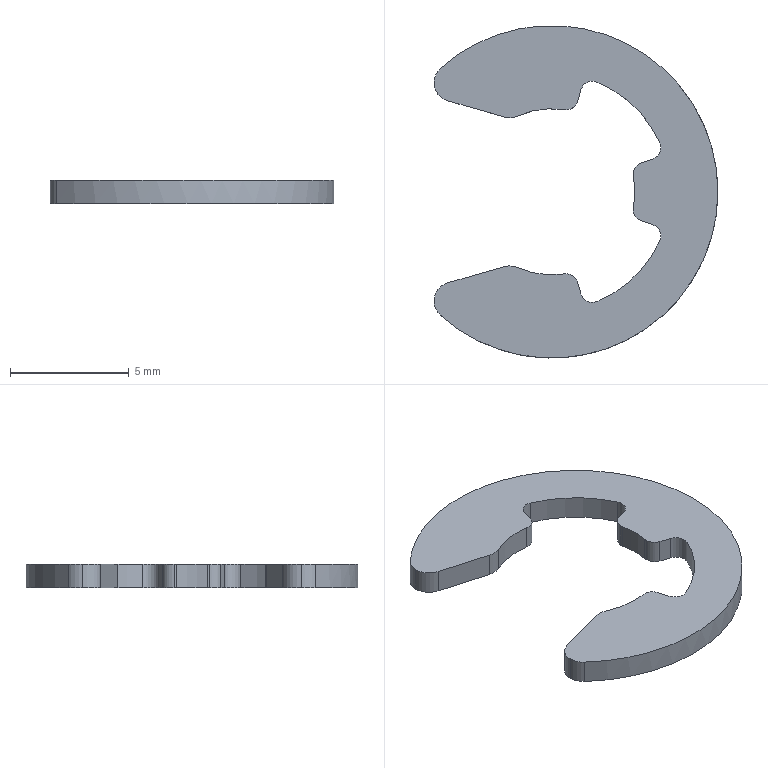Part | STEP file | MSBR-21_1_1_1_1 | 1 solid | 30 faces | box 11.954 x 14 x 1 mm | volume 73.77 mm3 | cylinder 22 | plane 8 | commonest cylinder face diameters 1 x10 1.6 x6 7 x3 10 x2 14 x1
STEP:
#1=CARTESIAN_POINT('',(0.,0.,0.));
#2=DIRECTION('',(0.,0.,1.));
#3=DIRECTION('',(1.,0.,0.));
#4=AXIS2_PLACEMENT_3D('',#1,#2,#3);
#5=CARTESIAN_POINT('',(3.438,0.657,29.2));
#6=VERTEX_POINT('',#5);
#7=CARTESIAN_POINT('',(3.438,-0.657,29.2));
#8=VERTEX_POINT('',#7);
#9=CARTESIAN_POINT('',(-0.000000002,0.000000005,29.2));
#10=DIRECTION('',(0.,0.,-1.));
#11=DIRECTION('',(0.9822,0.1877,0.));
#12=AXIS2_PLACEMENT_3D('',#9,#10,#11);
#13=CIRCLE('',#12,3.5);
#14=EDGE_CURVE('',#6,#8,#13,.T.);
#15=ORIENTED_EDGE('',*,*,#14,.T.);
#16=CARTESIAN_POINT('',(3.429,-0.7508,29.2));
#17=VERTEX_POINT('',#16);
#18=CARTESIAN_POINT('',(3.929,-0.7508,29.2));
#19=DIRECTION('',(0.,0.,1.));
#20=DIRECTION('',(-0.9822,0.1877,0.));
#21=AXIS2_PLACEMENT_3D('',#18,#19,#20);
#22=CIRCLE('',#21,0.5);
#23=EDGE_CURVE('',#8,#17,#22,.T.);
#24=ORIENTED_EDGE('',*,*,#23,.T.);
#25=CARTESIAN_POINT('',(3.774,-1.226,29.2));
#26=VERTEX_POINT('',#25);
#27=CARTESIAN_POINT('',(3.929,-0.7508,29.2));
#28=DIRECTION('',(0.,0.,1.));
#29=DIRECTION('',(-1.,-0.000000003,0.));
#30=AXIS2_PLACEMENT_3D('',#27,#28,#29);
#31=CIRCLE('',#30,0.5);
#32=EDGE_CURVE('',#17,#26,#31,.T.);
#33=ORIENTED_EDGE('',*,*,#32,.T.);
#34=CARTESIAN_POINT('',(4.253,-1.382,29.2));
#35=VERTEX_POINT('',#34);
#36=CARTESIAN_POINT('',(3.774,-1.226,29.2));
#37=DIRECTION('',(0.9511,-0.309,0.));
#38=VECTOR('',#37,0.5035);
#39=LINE('',#36,#38);
#40=EDGE_CURVE('',#26,#35,#39,.T.);
#41=ORIENTED_EDGE('',*,*,#40,.T.);
#42=CARTESIAN_POINT('',(4.554,-2.064,29.2));
#43=VERTEX_POINT('',#42);
#44=CARTESIAN_POINT('',(4.099,-1.857,29.2));
#45=DIRECTION('',(0.,0.,-1.));
#46=DIRECTION('',(0.309,0.9511,0.));
#47=AXIS2_PLACEMENT_3D('',#44,#45,#46);
#48=CIRCLE('',#47,0.5);
#49=EDGE_CURVE('',#35,#43,#48,.T.);
#50=ORIENTED_EDGE('',*,*,#49,.T.);
#51=CARTESIAN_POINT('',(1.904,-4.623,29.2));
#52=VERTEX_POINT('',#51);
#53=CARTESIAN_POINT('',(-0.000000006,0.000000006,29.2));
#54=DIRECTION('',(0.,0.,-1.));
#55=DIRECTION('',(0.9108,-0.4128,0.));
#56=AXIS2_PLACEMENT_3D('',#53,#54,#55);
#57=CIRCLE('',#56,5.);
#58=EDGE_CURVE('',#43,#52,#57,.T.);
#59=ORIENTED_EDGE('',*,*,#58,.T.);
#60=CARTESIAN_POINT('',(1.233,-4.299,29.2));
#61=VERTEX_POINT('',#60);
#62=CARTESIAN_POINT('',(1.713,-4.161,29.2));
#63=DIRECTION('',(0.,0.,-1.));
#64=DIRECTION('',(0.3807,-0.9247,0.));
#65=AXIS2_PLACEMENT_3D('',#62,#63,#64);
#66=CIRCLE('',#65,0.5);
#67=EDGE_CURVE('',#52,#61,#66,.T.);
#68=ORIENTED_EDGE('',*,*,#67,.T.);
#69=CARTESIAN_POINT('',(1.094,-3.815,29.2));
#70=VERTEX_POINT('',#69);
#71=CARTESIAN_POINT('',(1.233,-4.299,29.2));
#72=DIRECTION('',(-0.2756,0.9613,0.));
#73=VECTOR('',#72,0.5035);
#74=LINE('',#71,#73);
#75=EDGE_CURVE('',#61,#70,#74,.T.);
#76=ORIENTED_EDGE('',*,*,#75,.T.);
#77=CARTESIAN_POINT('',(0.5366,-3.459,29.2));
#78=VERTEX_POINT('',#77);
#79=CARTESIAN_POINT('',(0.6133,-3.953,29.2));
#80=DIRECTION('',(0.,0.,1.));
#81=DIRECTION('',(0.9613,0.2756,0.));
#82=AXIS2_PLACEMENT_3D('',#79,#80,#81);
#83=CIRCLE('',#82,0.5);
#84=EDGE_CURVE('',#70,#78,#83,.T.);
#85=ORIENTED_EDGE('',*,*,#84,.T.);
#86=CARTESIAN_POINT('',(-1.44,-3.19,29.2));
#87=VERTEX_POINT('',#86);
#88=CARTESIAN_POINT('',(-0.000000004,0.000000014,29.2));
#89=DIRECTION('',(0.,0.,-1.));
#90=DIRECTION('',(0.1533,-0.9882,0.));
#91=AXIS2_PLACEMENT_3D('',#88,#89,#90);
#92=CIRCLE('',#91,3.5);
#93=EDGE_CURVE('',#78,#87,#92,.T.);
#94=ORIENTED_EDGE('',*,*,#93,.T.);
#95=CARTESIAN_POINT('',(-1.99,-3.15,29.2));
#96=VERTEX_POINT('',#95);
#97=CARTESIAN_POINT('',(-1.77,-3.919,29.2));
#98=DIRECTION('',(0.,0.,1.));
#99=DIRECTION('',(0.4115,0.9114,0.));
#100=AXIS2_PLACEMENT_3D('',#97,#98,#99);
#101=CIRCLE('',#100,0.8);
#102=EDGE_CURVE('',#87,#96,#101,.T.);
#103=ORIENTED_EDGE('',*,*,#102,.T.);
#104=CARTESIAN_POINT('',(-4.374,-3.834,29.2));
#105=VERTEX_POINT('',#104);
#106=CARTESIAN_POINT('',(-1.99,-3.15,29.2));
#107=DIRECTION('',(-0.9613,-0.2756,0.));
#108=VECTOR('',#107,2.48);
#109=LINE('',#106,#108);
#110=EDGE_CURVE('',#96,#105,#109,.T.);
#111=ORIENTED_EDGE('',*,*,#110,.T.);
#112=CARTESIAN_POINT('',(-4.954,-4.603,29.2));
#113=VERTEX_POINT('',#112);
#114=CARTESIAN_POINT('',(-4.154,-4.603,29.2));
#115=DIRECTION('',(0.,0.,1.));
#116=DIRECTION('',(-0.2756,0.9613,0.));
#117=AXIS2_PLACEMENT_3D('',#114,#115,#116);
#118=CIRCLE('',#117,0.8);
#119=EDGE_CURVE('',#105,#113,#118,.T.);
#120=ORIENTED_EDGE('',*,*,#119,.T.);
#121=CARTESIAN_POINT('',(-4.69,-5.197,29.2));
#122=VERTEX_POINT('',#121);
#123=CARTESIAN_POINT('',(-4.154,-4.603,29.2));
#124=DIRECTION('',(0.,0.,1.));
#125=DIRECTION('',(-1.,0.000000001,0.));
#126=AXIS2_PLACEMENT_3D('',#123,#124,#125);
#127=CIRCLE('',#126,0.8);
#128=EDGE_CURVE('',#113,#122,#127,.T.);
#129=ORIENTED_EDGE('',*,*,#128,.T.);
#130=CARTESIAN_POINT('',(4.69,5.197,29.2));
#131=VERTEX_POINT('',#130);
#132=CARTESIAN_POINT('',(-0.000000007,0.000000005,29.2));
#133=DIRECTION('',(0.,0.,1.));
#134=DIRECTION('',(-0.67,-0.7424,0.));
#135=AXIS2_PLACEMENT_3D('',#132,#133,#134);
#136=CIRCLE('',#135,7.);
#137=EDGE_CURVE('',#122,#131,#136,.T.);
#138=ORIENTED_EDGE('',*,*,#137,.T.);
#139=CARTESIAN_POINT('',(-4.69,5.197,29.2));
#140=VERTEX_POINT('',#139);
#141=CARTESIAN_POINT('',(-0.000000007,0.000000005,29.2));
#142=DIRECTION('',(0.,0.,1.));
#143=DIRECTION('',(0.67,0.7424,0.));
#144=AXIS2_PLACEMENT_3D('',#141,#142,#143);
#145=CIRCLE('',#144,7.);
#146=EDGE_CURVE('',#131,#140,#145,.T.);
#147=ORIENTED_EDGE('',*,*,#146,.T.);
#148=CARTESIAN_POINT('',(-4.954,4.603,29.2));
#149=VERTEX_POINT('',#148);
#150=CARTESIAN_POINT('',(-4.154,4.603,29.2));
#151=DIRECTION('',(0.,0.,1.));
#152=DIRECTION('',(-0.67,0.7424,0.));
#153=AXIS2_PLACEMENT_3D('',#150,#151,#152);
#154=CIRCLE('',#153,0.8);
#155=EDGE_CURVE('',#140,#149,#154,.T.);
#156=ORIENTED_EDGE('',*,*,#155,.T.);
#157=CARTESIAN_POINT('',(-4.374,3.834,29.2));
#158=VERTEX_POINT('',#157);
#159=CARTESIAN_POINT('',(-4.154,4.603,29.2));
#160=DIRECTION('',(0.,0.,1.));
#161=DIRECTION('',(-1.,-0.000000001,0.));
#162=AXIS2_PLACEMENT_3D('',#159,#160,#161);
#163=CIRCLE('',#162,0.8);
#164=EDGE_CURVE('',#149,#158,#163,.T.);
#165=ORIENTED_EDGE('',*,*,#164,.T.);
#166=CARTESIAN_POINT('',(-1.99,3.15,29.2));
#167=VERTEX_POINT('',#166);
#168=CARTESIAN_POINT('',(-4.374,3.834,29.2));
#169=DIRECTION('',(0.9613,-0.2756,0.));
#170=VECTOR('',#169,2.48);
#171=LINE('',#168,#170);
#172=EDGE_CURVE('',#158,#167,#171,.T.);
#173=ORIENTED_EDGE('',*,*,#172,.T.);
#174=CARTESIAN_POINT('',(-1.44,3.19,29.2));
#175=VERTEX_POINT('',#174);
#176=CARTESIAN_POINT('',(-1.77,3.919,29.2));
#177=DIRECTION('',(0.,0.,1.));
#178=DIRECTION('',(-0.2756,-0.9613,0.));
#179=AXIS2_PLACEMENT_3D('',#176,#177,#178);
#180=CIRCLE('',#179,0.8);
#181=EDGE_CURVE('',#167,#175,#180,.T.);
#182=ORIENTED_EDGE('',*,*,#181,.T.);
#183=CARTESIAN_POINT('',(0.5366,3.459,29.2));
#184=VERTEX_POINT('',#183);
#185=CARTESIAN_POINT('',(-0.000000004,-0.000000004,29.2));
#186=DIRECTION('',(0.,0.,-1.));
#187=DIRECTION('',(-0.4115,0.9114,0.));
#188=AXIS2_PLACEMENT_3D('',#185,#186,#187);
#189=CIRCLE('',#188,3.5);
#190=EDGE_CURVE('',#175,#184,#189,.T.);
#191=ORIENTED_EDGE('',*,*,#190,.T.);
#192=CARTESIAN_POINT('',(1.094,3.815,29.2));
#193=VERTEX_POINT('',#192);
#194=CARTESIAN_POINT('',(0.6133,3.953,29.2));
#195=DIRECTION('',(0.,0.,1.));
#196=DIRECTION('',(-0.1533,-0.9882,0.));
#197=AXIS2_PLACEMENT_3D('',#194,#195,#196);
#198=CIRCLE('',#197,0.5);
#199=EDGE_CURVE('',#184,#193,#198,.T.);
#200=ORIENTED_EDGE('',*,*,#199,.T.);
#201=CARTESIAN_POINT('',(1.233,4.299,29.2));
#202=VERTEX_POINT('',#201);
#203=CARTESIAN_POINT('',(1.094,3.815,29.2));
#204=DIRECTION('',(0.2756,0.9613,0.));
#205=VECTOR('',#204,0.5035);
#206=LINE('',#203,#205);
#207=EDGE_CURVE('',#193,#202,#206,.T.);
#208=ORIENTED_EDGE('',*,*,#207,.T.);
#209=CARTESIAN_POINT('',(1.904,4.623,29.2));
#210=VERTEX_POINT('',#209);
#211=CARTESIAN_POINT('',(1.713,4.161,29.2));
#212=DIRECTION('',(0.,0.,-1.));
#213=DIRECTION('',(-0.9613,0.2756,0.));
#214=AXIS2_PLACEMENT_3D('',#211,#212,#213);
#215=CIRCLE('',#214,0.5);
#216=EDGE_CURVE('',#202,#210,#215,.T.);
#217=ORIENTED_EDGE('',*,*,#216,.T.);
#218=CARTESIAN_POINT('',(4.554,2.064,29.2));
#219=VERTEX_POINT('',#218);
#220=CARTESIAN_POINT('',(-0.000000006,0.000000004,29.2));
#221=DIRECTION('',(0.,0.,-1.));
#222=DIRECTION('',(0.3807,0.9247,0.));
#223=AXIS2_PLACEMENT_3D('',#220,#221,#222);
#224=CIRCLE('',#223,5.);
#225=EDGE_CURVE('',#210,#219,#224,.T.);
#226=ORIENTED_EDGE('',*,*,#225,.T.);
#227=CARTESIAN_POINT('',(4.253,1.382,29.2));
#228=VERTEX_POINT('',#227);
#229=CARTESIAN_POINT('',(4.099,1.857,29.2));
#230=DIRECTION('',(0.,0.,-1.));
#231=DIRECTION('',(0.9108,0.4128,0.));
#232=AXIS2_PLACEMENT_3D('',#229,#230,#231);
#233=CIRCLE('',#232,0.5);
#234=EDGE_CURVE('',#219,#228,#233,.T.);
#235=ORIENTED_EDGE('',*,*,#234,.T.);
#236=CARTESIAN_POINT('',(3.774,1.226,29.2));
#237=VERTEX_POINT('',#236);
#238=CARTESIAN_POINT('',(4.253,1.382,29.2));
#239=DIRECTION('',(-0.9511,-0.309,0.));
#240=VECTOR('',#239,0.5035);
#241=LINE('',#238,#240);
#242=EDGE_CURVE('',#228,#237,#241,.T.);
#243=ORIENTED_EDGE('',*,*,#242,.T.);
#244=CARTESIAN_POINT('',(3.429,0.7508,29.2));
#245=VERTEX_POINT('',#244);
#246=CARTESIAN_POINT('',(3.929,0.7508,29.2));
#247=DIRECTION('',(0.,0.,1.));
#248=DIRECTION('',(-0.309,0.9511,0.));
#249=AXIS2_PLACEMENT_3D('',#246,#247,#248);
#250=CIRCLE('',#249,0.5);
#251=EDGE_CURVE('',#237,#245,#250,.T.);
#252=ORIENTED_EDGE('',*,*,#251,.T.);
#253=CARTESIAN_POINT('',(3.929,0.7508,29.2));
#254=DIRECTION('',(0.,0.,1.));
#255=DIRECTION('',(-1.,-0.000000007,0.));
#256=AXIS2_PLACEMENT_3D('',#253,#254,#255);
#257=CIRCLE('',#256,0.5);
#258=EDGE_CURVE('',#245,#6,#257,.T.);
#259=ORIENTED_EDGE('',*,*,#258,.T.);
#260=EDGE_LOOP('',(#15,#24,#33,#41,#50,#59,#68,#76,#85,#94,#103,#111,#120,#129,#138,#147,#156,#165,#173,#182,#191,#200,#208,#217,#226,#235,#243,#252,#259));
#261=FACE_OUTER_BOUND('',#260,.F.);
#262=CARTESIAN_POINT('',(1.025,0.000002085,29.2));
#263=DIRECTION('',(0.,0.,1.));
#264=DIRECTION('',(0.,1.,0.));
#265=AXIS2_PLACEMENT_3D('',#262,#263,#264);
#266=PLANE('',#265);
#267=ADVANCED_FACE('',(#261),#266,.F.);
#268=CARTESIAN_POINT('',(3.438,-0.657,30.2));
#269=VERTEX_POINT('',#268);
#270=CARTESIAN_POINT('',(3.438,0.657,30.2));
#271=VERTEX_POINT('',#270);
#272=CARTESIAN_POINT('',(-0.000000002,0.000000005,30.2));
#273=DIRECTION('',(0.,0.,1.));
#274=DIRECTION('',(0.9822,-0.1877,0.));
#275=AXIS2_PLACEMENT_3D('',#272,#273,#274);
#276=CIRCLE('',#275,3.5);
#277=EDGE_CURVE('',#269,#271,#276,.T.);
#278=ORIENTED_EDGE('',*,*,#277,.F.);
#279=CARTESIAN_POINT('',(3.438,-0.657,29.2));
#280=DIRECTION('',(0.,0.,1.));
#281=VECTOR('',#280,1.);
#282=LINE('',#279,#281);
#283=EDGE_CURVE('',#8,#269,#282,.T.);
#284=ORIENTED_EDGE('',*,*,#283,.F.);
#285=ORIENTED_EDGE('',*,*,#14,.F.);
#286=CARTESIAN_POINT('',(3.438,0.657,30.2));
#287=DIRECTION('',(0.,0.,-1.));
#288=VECTOR('',#287,1.);
#289=LINE('',#286,#288);
#290=EDGE_CURVE('',#271,#6,#289,.T.);
#291=ORIENTED_EDGE('',*,*,#290,.F.);
#292=EDGE_LOOP('',(#278,#284,#285,#291));
#293=FACE_OUTER_BOUND('',#292,.F.);
#294=CARTESIAN_POINT('',(-0.000000002,0.000000005,29.178));
#295=DIRECTION('',(0.,0.,1.));
#296=DIRECTION('',(0.9822,-0.1877,0.));
#297=AXIS2_PLACEMENT_3D('',#294,#295,#296);
#298=CYLINDRICAL_SURFACE('',#297,3.5);
#299=ADVANCED_FACE('',(#293),#298,.F.);
#300=CARTESIAN_POINT('',(4.253,-1.382,30.2));
#301=VERTEX_POINT('',#300);
#302=CARTESIAN_POINT('',(3.774,-1.226,30.2));
#303=VERTEX_POINT('',#302);
#304=CARTESIAN_POINT('',(4.253,-1.382,30.2));
#305=DIRECTION('',(-0.9511,0.309,0.));
#306=VECTOR('',#305,0.5035);
#307=LINE('',#304,#306);
#308=EDGE_CURVE('',#301,#303,#307,.T.);
#309=ORIENTED_EDGE('',*,*,#308,.T.);
#310=CARTESIAN_POINT('',(3.429,-0.7508,30.2));
#311=VERTEX_POINT('',#310);
#312=CARTESIAN_POINT('',(3.929,-0.7508,30.2));
#313=DIRECTION('',(0.,0.,-1.));
#314=DIRECTION('',(-0.309,-0.9511,0.));
#315=AXIS2_PLACEMENT_3D('',#312,#313,#314);
#316=CIRCLE('',#315,0.5);
#317=EDGE_CURVE('',#303,#311,#316,.T.);
#318=ORIENTED_EDGE('',*,*,#317,.T.);
#319=CARTESIAN_POINT('',(3.929,-0.7508,30.2));
#320=DIRECTION('',(0.,0.,-1.));
#321=DIRECTION('',(-1.,0.000000007,0.));
#322=AXIS2_PLACEMENT_3D('',#319,#320,#321);
#323=CIRCLE('',#322,0.5);
#324=EDGE_CURVE('',#311,#269,#323,.T.);
#325=ORIENTED_EDGE('',*,*,#324,.T.);
#326=ORIENTED_EDGE('',*,*,#277,.T.);
#327=CARTESIAN_POINT('',(3.429,0.7508,30.2));
#328=VERTEX_POINT('',#327);
#329=CARTESIAN_POINT('',(3.929,0.7508,30.2));
#330=DIRECTION('',(0.,0.,-1.));
#331=DIRECTION('',(-0.9822,-0.1877,0.));
#332=AXIS2_PLACEMENT_3D('',#329,#330,#331);
#333=CIRCLE('',#332,0.5);
#334=EDGE_CURVE('',#271,#328,#333,.T.);
#335=ORIENTED_EDGE('',*,*,#334,.T.);
#336=CARTESIAN_POINT('',(3.774,1.226,30.2));
#337=VERTEX_POINT('',#336);
#338=CARTESIAN_POINT('',(3.929,0.7508,30.2));
#339=DIRECTION('',(0.,0.,-1.));
#340=DIRECTION('',(-1.,0.000000003,0.));
#341=AXIS2_PLACEMENT_3D('',#338,#339,#340);
#342=CIRCLE('',#341,0.5);
#343=EDGE_CURVE('',#328,#337,#342,.T.);
#344=ORIENTED_EDGE('',*,*,#343,.T.);
#345=CARTESIAN_POINT('',(4.253,1.382,30.2));
#346=VERTEX_POINT('',#345);
#347=CARTESIAN_POINT('',(3.774,1.226,30.2));
#348=DIRECTION('',(0.9511,0.309,0.));
#349=VECTOR('',#348,0.5035);
#350=LINE('',#347,#349);
#351=EDGE_CURVE('',#337,#346,#350,.T.);
#352=ORIENTED_EDGE('',*,*,#351,.T.);
#353=CARTESIAN_POINT('',(4.554,2.064,30.2));
#354=VERTEX_POINT('',#353);
#355=CARTESIAN_POINT('',(4.099,1.857,30.2));
#356=DIRECTION('',(0.,0.,1.));
#357=DIRECTION('',(0.309,-0.9511,0.));
#358=AXIS2_PLACEMENT_3D('',#355,#356,#357);
#359=CIRCLE('',#358,0.5);
#360=EDGE_CURVE('',#346,#354,#359,.T.);
#361=ORIENTED_EDGE('',*,*,#360,.T.);
#362=CARTESIAN_POINT('',(1.904,4.623,30.2));
#363=VERTEX_POINT('',#362);
#364=CARTESIAN_POINT('',(-0.000000006,0.000000004,30.2));
#365=DIRECTION('',(0.,0.,1.));
#366=DIRECTION('',(0.9108,0.4128,0.));
#367=AXIS2_PLACEMENT_3D('',#364,#365,#366);
#368=CIRCLE('',#367,5.);
#369=EDGE_CURVE('',#354,#363,#368,.T.);
#370=ORIENTED_EDGE('',*,*,#369,.T.);
#371=CARTESIAN_POINT('',(1.233,4.299,30.2));
#372=VERTEX_POINT('',#371);
#373=CARTESIAN_POINT('',(1.713,4.161,30.2));
#374=DIRECTION('',(0.,0.,1.));
#375=DIRECTION('',(0.3807,0.9247,0.));
#376=AXIS2_PLACEMENT_3D('',#373,#374,#375);
#377=CIRCLE('',#376,0.5);
#378=EDGE_CURVE('',#363,#372,#377,.T.);
#379=ORIENTED_EDGE('',*,*,#378,.T.);
#380=CARTESIAN_POINT('',(1.094,3.815,30.2));
#381=VERTEX_POINT('',#380);
#382=CARTESIAN_POINT('',(1.233,4.299,30.2));
#383=DIRECTION('',(-0.2756,-0.9613,0.));
#384=VECTOR('',#383,0.5035);
#385=LINE('',#382,#384);
#386=EDGE_CURVE('',#372,#381,#385,.T.);
#387=ORIENTED_EDGE('',*,*,#386,.T.);
#388=CARTESIAN_POINT('',(0.5366,3.459,30.2));
#389=VERTEX_POINT('',#388);
#390=CARTESIAN_POINT('',(0.6133,3.953,30.2));
#391=DIRECTION('',(0.,0.,-1.));
#392=DIRECTION('',(0.9613,-0.2756,0.));
#393=AXIS2_PLACEMENT_3D('',#390,#391,#392);
#394=CIRCLE('',#393,0.5);
#395=EDGE_CURVE('',#381,#389,#394,.T.);
#396=ORIENTED_EDGE('',*,*,#395,.T.);
#397=CARTESIAN_POINT('',(-1.44,3.19,30.2));
#398=VERTEX_POINT('',#397);
#399=CARTESIAN_POINT('',(-0.000000004,-0.000000004,30.2));
#400=DIRECTION('',(0.,0.,1.));
#401=DIRECTION('',(0.1533,0.9882,0.));
#402=AXIS2_PLACEMENT_3D('',#399,#400,#401);
#403=CIRCLE('',#402,3.5);
#404=EDGE_CURVE('',#389,#398,#403,.T.);
#405=ORIENTED_EDGE('',*,*,#404,.T.);
#406=CARTESIAN_POINT('',(-1.99,3.15,30.2));
#407=VERTEX_POINT('',#406);
#408=CARTESIAN_POINT('',(-1.77,3.919,30.2));
#409=DIRECTION('',(0.,0.,-1.));
#410=DIRECTION('',(0.4115,-0.9114,0.));
#411=AXIS2_PLACEMENT_3D('',#408,#409,#410);
#412=CIRCLE('',#411,0.8);
#413=EDGE_CURVE('',#398,#407,#412,.T.);
#414=ORIENTED_EDGE('',*,*,#413,.T.);
#415=CARTESIAN_POINT('',(-4.374,3.834,30.2));
#416=VERTEX_POINT('',#415);
#417=CARTESIAN_POINT('',(-1.99,3.15,30.2));
#418=DIRECTION('',(-0.9613,0.2756,0.));
#419=VECTOR('',#418,2.48);
#420=LINE('',#417,#419);
#421=EDGE_CURVE('',#407,#416,#420,.T.);
#422=ORIENTED_EDGE('',*,*,#421,.T.);
#423=CARTESIAN_POINT('',(-4.954,4.603,30.2));
#424=VERTEX_POINT('',#423);
#425=CARTESIAN_POINT('',(-4.154,4.603,30.2));
#426=DIRECTION('',(0.,0.,-1.));
#427=DIRECTION('',(-0.2756,-0.9613,0.));
#428=AXIS2_PLACEMENT_3D('',#425,#426,#427);
#429=CIRCLE('',#428,0.8);
#430=EDGE_CURVE('',#416,#424,#429,.T.);
#431=ORIENTED_EDGE('',*,*,#430,.T.);
#432=CARTESIAN_POINT('',(-4.69,5.197,30.2));
#433=VERTEX_POINT('',#432);
#434=CARTESIAN_POINT('',(-4.154,4.603,30.2));
#435=DIRECTION('',(0.,0.,-1.));
#436=DIRECTION('',(-1.,-0.000000001,0.));
#437=AXIS2_PLACEMENT_3D('',#434,#435,#436);
#438=CIRCLE('',#437,0.8);
#439=EDGE_CURVE('',#424,#433,#438,.T.);
#440=ORIENTED_EDGE('',*,*,#439,.T.);
#441=CARTESIAN_POINT('',(4.69,5.197,30.2));
#442=VERTEX_POINT('',#441);
#443=CARTESIAN_POINT('',(-0.000000007,0.000000005,30.2));
#444=DIRECTION('',(0.,0.,-1.));
#445=DIRECTION('',(-0.67,0.7424,0.));
#446=AXIS2_PLACEMENT_3D('',#443,#444,#445);
#447=CIRCLE('',#446,7.);
#448=EDGE_CURVE('',#433,#442,#447,.T.);
#449=ORIENTED_EDGE('',*,*,#448,.T.);
#450=CARTESIAN_POINT('',(4.69,-5.197,30.2));
#451=VERTEX_POINT('',#450);
#452=CARTESIAN_POINT('',(-0.000000007,0.000000005,30.2));
#453=DIRECTION('',(0.,0.,-1.));
#454=DIRECTION('',(0.67,0.7424,0.));
#455=AXIS2_PLACEMENT_3D('',#452,#453,#454);
#456=CIRCLE('',#455,7.);
#457=EDGE_CURVE('',#442,#451,#456,.T.);
#458=ORIENTED_EDGE('',*,*,#457,.T.);
#459=CARTESIAN_POINT('',(-4.69,-5.197,30.2));
#460=VERTEX_POINT('',#459);
#461=CARTESIAN_POINT('',(-0.000000007,0.000000005,30.2));
#462=DIRECTION('',(0.,0.,-1.));
#463=DIRECTION('',(0.67,-0.7424,0.));
#464=AXIS2_PLACEMENT_3D('',#461,#462,#463);
#465=CIRCLE('',#464,7.);
#466=EDGE_CURVE('',#451,#460,#465,.T.);
#467=ORIENTED_EDGE('',*,*,#466,.T.);
#468=CARTESIAN_POINT('',(-4.954,-4.603,30.2));
#469=VERTEX_POINT('',#468);
#470=CARTESIAN_POINT('',(-4.154,-4.603,30.2));
#471=DIRECTION('',(0.,0.,-1.));
#472=DIRECTION('',(-0.67,-0.7424,0.));
#473=AXIS2_PLACEMENT_3D('',#470,#471,#472);
#474=CIRCLE('',#473,0.8);
#475=EDGE_CURVE('',#460,#469,#474,.T.);
#476=ORIENTED_EDGE('',*,*,#475,.T.);
#477=CARTESIAN_POINT('',(-4.374,-3.834,30.2));
#478=VERTEX_POINT('',#477);
#479=CARTESIAN_POINT('',(-4.154,-4.603,30.2));
#480=DIRECTION('',(0.,0.,-1.));
#481=DIRECTION('',(-1.,0.000000001,0.));
#482=AXIS2_PLACEMENT_3D('',#479,#480,#481);
#483=CIRCLE('',#482,0.8);
#484=EDGE_CURVE('',#469,#478,#483,.T.);
#485=ORIENTED_EDGE('',*,*,#484,.T.);
#486=CARTESIAN_POINT('',(-1.99,-3.15,30.2));
#487=VERTEX_POINT('',#486);
#488=CARTESIAN_POINT('',(-4.374,-3.834,30.2));
#489=DIRECTION('',(0.9613,0.2756,0.));
#490=VECTOR('',#489,2.48);
#491=LINE('',#488,#490);
#492=EDGE_CURVE('',#478,#487,#491,.T.);
#493=ORIENTED_EDGE('',*,*,#492,.T.);
#494=CARTESIAN_POINT('',(-1.44,-3.19,30.2));
#495=VERTEX_POINT('',#494);
#496=CARTESIAN_POINT('',(-1.77,-3.919,30.2));
#497=DIRECTION('',(0.,0.,-1.));
#498=DIRECTION('',(-0.2756,0.9613,0.));
#499=AXIS2_PLACEMENT_3D('',#496,#497,#498);
#500=CIRCLE('',#499,0.8);
#501=EDGE_CURVE('',#487,#495,#500,.T.);
#502=ORIENTED_EDGE('',*,*,#501,.T.);
#503=CARTESIAN_POINT('',(0.5366,-3.459,30.2));
#504=VERTEX_POINT('',#503);
#505=CARTESIAN_POINT('',(-0.000000004,0.000000014,30.2));
#506=DIRECTION('',(0.,0.,1.));
#507=DIRECTION('',(-0.4115,-0.9114,0.));
#508=AXIS2_PLACEMENT_3D('',#505,#506,#507);
#509=CIRCLE('',#508,3.5);
#510=EDGE_CURVE('',#495,#504,#509,.T.);
#511=ORIENTED_EDGE('',*,*,#510,.T.);
#512=CARTESIAN_POINT('',(1.094,-3.815,30.2));
#513=VERTEX_POINT('',#512);
#514=CARTESIAN_POINT('',(0.6133,-3.953,30.2));
#515=DIRECTION('',(0.,0.,-1.));
#516=DIRECTION('',(-0.1533,0.9882,0.));
#517=AXIS2_PLACEMENT_3D('',#514,#515,#516);
#518=CIRCLE('',#517,0.5);
#519=EDGE_CURVE('',#504,#513,#518,.T.);
#520=ORIENTED_EDGE('',*,*,#519,.T.);
#521=CARTESIAN_POINT('',(1.233,-4.299,30.2));
#522=VERTEX_POINT('',#521);
#523=CARTESIAN_POINT('',(1.094,-3.815,30.2));
#524=DIRECTION('',(0.2756,-0.9613,0.));
#525=VECTOR('',#524,0.5035);
#526=LINE('',#523,#525);
#527=EDGE_CURVE('',#513,#522,#526,.T.);
#528=ORIENTED_EDGE('',*,*,#527,.T.);
#529=CARTESIAN_POINT('',(1.904,-4.623,30.2));
#530=VERTEX_POINT('',#529);
#531=CARTESIAN_POINT('',(1.713,-4.161,30.2));
#532=DIRECTION('',(0.,0.,1.));
#533=DIRECTION('',(-0.9613,-0.2756,0.));
#534=AXIS2_PLACEMENT_3D('',#531,#532,#533);
#535=CIRCLE('',#534,0.5);
#536=EDGE_CURVE('',#522,#530,#535,.T.);
#537=ORIENTED_EDGE('',*,*,#536,.T.);
#538=CARTESIAN_POINT('',(4.554,-2.064,30.2));
#539=VERTEX_POINT('',#538);
#540=CARTESIAN_POINT('',(-0.000000006,0.000000006,30.2));
#541=DIRECTION('',(0.,0.,1.));
#542=DIRECTION('',(0.3807,-0.9247,0.));
#543=AXIS2_PLACEMENT_3D('',#540,#541,#542);
#544=CIRCLE('',#543,5.);
#545=EDGE_CURVE('',#530,#539,#544,.T.);
#546=ORIENTED_EDGE('',*,*,#545,.T.);
#547=CARTESIAN_POINT('',(4.099,-1.857,30.2));
#548=DIRECTION('',(0.,0.,1.));
#549=DIRECTION('',(0.9108,-0.4128,0.));
#550=AXIS2_PLACEMENT_3D('',#547,#548,#549);
#551=CIRCLE('',#550,0.5);
#552=EDGE_CURVE('',#539,#301,#551,.T.);
#553=ORIENTED_EDGE('',*,*,#552,.T.);
#554=EDGE_LOOP('',(#309,#318,#325,#326,#335,#344,#352,#361,#370,#379,#387,#396,#405,#414,#422,#431,#440,#449,#458,#467,#476,#485,#493,#502,#511,#520,#528,#537,#546,#553));
#555=FACE_OUTER_BOUND('',#554,.F.);
#556=CARTESIAN_POINT('',(1.025,-0.000002076,30.2));
#557=DIRECTION('',(0.,0.,1.));
#558=DIRECTION('',(0.,1.,0.));
#559=AXIS2_PLACEMENT_3D('',#556,#557,#558);
#560=PLANE('',#559);
#561=ADVANCED_FACE('',(#555),#560,.T.);
#562=ORIENTED_EDGE('',*,*,#40,.F.);
#563=CARTESIAN_POINT('',(3.774,-1.226,30.2));
#564=DIRECTION('',(0.000000001,0.,-1.));
#565=VECTOR('',#564,1.);
#566=LINE('',#563,#565);
#567=EDGE_CURVE('',#303,#26,#566,.T.);
#568=ORIENTED_EDGE('',*,*,#567,.F.);
#569=ORIENTED_EDGE('',*,*,#308,.F.);
#570=CARTESIAN_POINT('',(4.253,-1.382,29.2));
#571=DIRECTION('',(0.,0.,1.));
#572=VECTOR('',#571,1.);
#573=LINE('',#570,#572);
#574=EDGE_CURVE('',#35,#301,#573,.T.);
#575=ORIENTED_EDGE('',*,*,#574,.F.);
#576=EDGE_LOOP('',(#562,#568,#569,#575));
#577=FACE_OUTER_BOUND('',#576,.F.);
#578=CARTESIAN_POINT('',(4.014,-1.304,29.7));
#579=DIRECTION('',(0.309,0.9511,0.));
#580=DIRECTION('',(0.9511,-0.309,0.));
#581=AXIS2_PLACEMENT_3D('',#578,#579,#580);
#582=PLANE('',#581);
#583=ADVANCED_FACE('',(#577),#582,.F.);
#584=ORIENTED_EDGE('',*,*,#567,.T.);
#585=ORIENTED_EDGE('',*,*,#32,.F.);
#586=CARTESIAN_POINT('',(3.429,-0.7508,30.2));
#587=DIRECTION('',(0.,0.,-1.));
#588=VECTOR('',#587,1.);
#589=LINE('',#586,#588);
#590=EDGE_CURVE('',#311,#17,#589,.T.);
#591=ORIENTED_EDGE('',*,*,#590,.F.);
#592=ORIENTED_EDGE('',*,*,#317,.F.);
#593=EDGE_LOOP('',(#584,#585,#591,#592));
#594=FACE_OUTER_BOUND('',#593,.F.);
#595=CARTESIAN_POINT('',(3.929,-0.7508,29.178));
#596=DIRECTION('',(0.,0.,1.));
#597=DIRECTION('',(-1.,-0.000000002,0.));
#598=AXIS2_PLACEMENT_3D('',#595,#596,#597);
#599=CYLINDRICAL_SURFACE('',#598,0.5);
#600=ADVANCED_FACE('',(#594),#599,.T.);
#601=ORIENTED_EDGE('',*,*,#324,.F.);
#602=ORIENTED_EDGE('',*,*,#590,.T.);
#603=ORIENTED_EDGE('',*,*,#23,.F.);
#604=ORIENTED_EDGE('',*,*,#283,.T.);
#605=EDGE_LOOP('',(#601,#602,#603,#604));
#606=FACE_OUTER_BOUND('',#605,.F.);
#607=CARTESIAN_POINT('',(3.929,-0.7508,29.178));
#608=DIRECTION('',(0.,0.,1.));
#609=DIRECTION('',(-0.9822,0.1877,0.));
#610=AXIS2_PLACEMENT_3D('',#607,#608,#609);
#611=CYLINDRICAL_SURFACE('',#610,0.5);
#612=ADVANCED_FACE('',(#606),#611,.T.);
#613=ORIENTED_EDGE('',*,*,#552,.F.);
#614=CARTESIAN_POINT('',(4.554,-2.064,29.2));
#615=DIRECTION('',(0.,0.,1.));
#616=VECTOR('',#615,1.);
#617=LINE('',#614,#616);
#618=EDGE_CURVE('',#43,#539,#617,.T.);
#619=ORIENTED_EDGE('',*,*,#618,.F.);
#620=ORIENTED_EDGE('',*,*,#49,.F.);
#621=ORIENTED_EDGE('',*,*,#574,.T.);
#622=EDGE_LOOP('',(#613,#619,#620,#621));
#623=FACE_OUTER_BOUND('',#622,.F.);
#624=CARTESIAN_POINT('',(4.099,-1.857,29.178));
#625=DIRECTION('',(0.,0.,1.));
#626=DIRECTION('',(0.9108,-0.4128,0.));
#627=AXIS2_PLACEMENT_3D('',#624,#625,#626);
#628=CYLINDRICAL_SURFACE('',#627,0.5);
#629=ADVANCED_FACE('',(#623),#628,.F.);
#630=ORIENTED_EDGE('',*,*,#545,.F.);
#631=CARTESIAN_POINT('',(1.904,-4.623,29.2));
#632=DIRECTION('',(0.,0.,1.));
#633=VECTOR('',#632,1.);
#634=LINE('',#631,#633);
#635=EDGE_CURVE('',#52,#530,#634,.T.);
#636=ORIENTED_EDGE('',*,*,#635,.F.);
#637=ORIENTED_EDGE('',*,*,#58,.F.);
#638=ORIENTED_EDGE('',*,*,#618,.T.);
#639=EDGE_LOOP('',(#630,#636,#637,#638));
#640=FACE_OUTER_BOUND('',#639,.F.);
#641=CARTESIAN_POINT('',(-0.000000006,0.000000006,29.178));
#642=DIRECTION('',(0.,0.,1.));
#643=DIRECTION('',(0.3807,-0.9247,0.));
#644=AXIS2_PLACEMENT_3D('',#641,#642,#643);
#645=CYLINDRICAL_SURFACE('',#644,5.);
#646=ADVANCED_FACE('',(#640),#645,.F.);
#647=ORIENTED_EDGE('',*,*,#536,.F.);
#648=CARTESIAN_POINT('',(1.233,-4.299,30.2));
#649=DIRECTION('',(0.,0.,-1.));
#650=VECTOR('',#649,1.);
#651=LINE('',#648,#650);
#652=EDGE_CURVE('',#522,#61,#651,.T.);
#653=ORIENTED_EDGE('',*,*,#652,.T.);
#654=ORIENTED_EDGE('',*,*,#67,.F.);
#655=ORIENTED_EDGE('',*,*,#635,.T.);
#656=EDGE_LOOP('',(#647,#653,#654,#655));
#657=FACE_OUTER_BOUND('',#656,.F.);
#658=CARTESIAN_POINT('',(1.713,-4.161,29.178));
#659=DIRECTION('',(0.,0.,1.));
#660=DIRECTION('',(-0.9613,-0.2756,0.));
#661=AXIS2_PLACEMENT_3D('',#658,#659,#660);
#662=CYLINDRICAL_SURFACE('',#661,0.5);
#663=ADVANCED_FACE('',(#657),#662,.F.);
#664=ORIENTED_EDGE('',*,*,#75,.F.);
#665=ORIENTED_EDGE('',*,*,#652,.F.);
#666=ORIENTED_EDGE('',*,*,#527,.F.);
#667=CARTESIAN_POINT('',(1.094,-3.815,29.2));
#668=DIRECTION('',(0.,0.,1.));
#669=VECTOR('',#668,1.);
#670=LINE('',#667,#669);
#671=EDGE_CURVE('',#70,#513,#670,.T.);
#672=ORIENTED_EDGE('',*,*,#671,.F.);
#673=EDGE_LOOP('',(#664,#665,#666,#672));
#674=FACE_OUTER_BOUND('',#673,.F.);
#675=CARTESIAN_POINT('',(1.163,-4.057,29.7));
#676=DIRECTION('',(0.9613,0.2756,0.));
#677=DIRECTION('',(-0.2756,0.9613,0.));
#678=AXIS2_PLACEMENT_3D('',#675,#676,#677);
#679=PLANE('',#678);
#680=ADVANCED_FACE('',(#674),#679,.T.);
#681=ORIENTED_EDGE('',*,*,#84,.F.);
#682=ORIENTED_EDGE('',*,*,#671,.T.);
#683=ORIENTED_EDGE('',*,*,#519,.F.);
#684=CARTESIAN_POINT('',(0.5366,-3.459,29.2));
#685=DIRECTION('',(0.,0.,1.));
#686=VECTOR('',#685,1.);
#687=LINE('',#684,#686);
#688=EDGE_CURVE('',#78,#504,#687,.T.);
#689=ORIENTED_EDGE('',*,*,#688,.F.);
#690=EDGE_LOOP('',(#681,#682,#683,#689));
#691=FACE_OUTER_BOUND('',#690,.F.);
#692=CARTESIAN_POINT('',(0.6133,-3.953,29.178));
#693=DIRECTION('',(0.,0.,1.));
#694=DIRECTION('',(0.9613,0.2756,0.));
#695=AXIS2_PLACEMENT_3D('',#692,#693,#694);
#696=CYLINDRICAL_SURFACE('',#695,0.5);
#697=ADVANCED_FACE('',(#691),#696,.T.);
#698=ORIENTED_EDGE('',*,*,#510,.F.);
#699=CARTESIAN_POINT('',(-1.44,-3.19,29.2));
#700=DIRECTION('',(0.,0.,1.));
#701=VECTOR('',#700,1.);
#702=LINE('',#699,#701);
#703=EDGE_CURVE('',#87,#495,#702,.T.);
#704=ORIENTED_EDGE('',*,*,#703,.F.);
#705=ORIENTED_EDGE('',*,*,#93,.F.);
#706=ORIENTED_EDGE('',*,*,#688,.T.);
#707=EDGE_LOOP('',(#698,#704,#705,#706));
#708=FACE_OUTER_BOUND('',#707,.F.);
#709=CARTESIAN_POINT('',(-0.000000004,0.000000014,29.178));
#710=DIRECTION('',(0.,0.,1.));
#711=DIRECTION('',(-0.4115,-0.9114,0.));
#712=AXIS2_PLACEMENT_3D('',#709,#710,#711);
#713=CYLINDRICAL_SURFACE('',#712,3.5);
#714=ADVANCED_FACE('',(#708),#713,.F.);
#715=ORIENTED_EDGE('',*,*,#102,.F.);
#716=ORIENTED_EDGE('',*,*,#703,.T.);
#717=ORIENTED_EDGE('',*,*,#501,.F.);
#718=CARTESIAN_POINT('',(-1.99,-3.15,30.2));
#719=DIRECTION('',(0.,0.,-1.));
#720=VECTOR('',#719,1.);
#721=LINE('',#718,#720);
#722=EDGE_CURVE('',#487,#96,#721,.T.);
#723=ORIENTED_EDGE('',*,*,#722,.T.);
#724=EDGE_LOOP('',(#715,#716,#717,#723));
#725=FACE_OUTER_BOUND('',#724,.F.);
#726=CARTESIAN_POINT('',(-1.77,-3.919,29.178));
#727=DIRECTION('',(0.,0.,1.));
#728=DIRECTION('',(0.4115,0.9114,0.));
#729=AXIS2_PLACEMENT_3D('',#726,#727,#728);
#730=CYLINDRICAL_SURFACE('',#729,0.8);
#731=ADVANCED_FACE('',(#725),#730,.T.);
#732=ORIENTED_EDGE('',*,*,#110,.F.);
#733=ORIENTED_EDGE('',*,*,#722,.F.);
#734=ORIENTED_EDGE('',*,*,#492,.F.);
#735=CARTESIAN_POINT('',(-4.374,-3.834,29.2));
#736=DIRECTION('',(0.,0.,1.));
#737=VECTOR('',#736,1.);
#738=LINE('',#735,#737);
#739=EDGE_CURVE('',#105,#478,#738,.T.);
#740=ORIENTED_EDGE('',*,*,#739,.F.);
#741=EDGE_LOOP('',(#732,#733,#734,#740));
#742=FACE_OUTER_BOUND('',#741,.F.);
#743=CARTESIAN_POINT('',(-3.182,-3.492,29.7));
#744=DIRECTION('',(-0.2756,0.9613,0.));
#745=DIRECTION('',(-0.9613,-0.2756,0.));
#746=AXIS2_PLACEMENT_3D('',#743,#744,#745);
#747=PLANE('',#746);
#748=ADVANCED_FACE('',(#742),#747,.T.);
#749=ORIENTED_EDGE('',*,*,#484,.F.);
#750=CARTESIAN_POINT('',(-4.954,-4.603,29.2));
#751=DIRECTION('',(0.,0.,1.));
#752=VECTOR('',#751,1.);
#753=LINE('',#750,#752);
#754=EDGE_CURVE('',#113,#469,#753,.T.);
#755=ORIENTED_EDGE('',*,*,#754,.F.);
#756=ORIENTED_EDGE('',*,*,#119,.F.);
#757=ORIENTED_EDGE('',*,*,#739,.T.);
#758=EDGE_LOOP('',(#749,#755,#756,#757));
#759=FACE_OUTER_BOUND('',#758,.F.);
#760=CARTESIAN_POINT('',(-4.154,-4.603,29.178));
#761=DIRECTION('',(0.,0.,1.));
#762=DIRECTION('',(-0.2756,0.9613,0.));
#763=AXIS2_PLACEMENT_3D('',#760,#761,#762);
#764=CYLINDRICAL_SURFACE('',#763,0.8);
#765=ADVANCED_FACE('',(#759),#764,.T.);
#766=CARTESIAN_POINT('',(-4.69,-5.197,29.2));
#767=DIRECTION('',(0.,0.,1.));
#768=VECTOR('',#767,1.);
#769=LINE('',#766,#768);
#770=EDGE_CURVE('',#122,#460,#769,.T.);
#771=ORIENTED_EDGE('',*,*,#770,.F.);
#772=ORIENTED_EDGE('',*,*,#128,.F.);
#773=ORIENTED_EDGE('',*,*,#754,.T.);
#774=ORIENTED_EDGE('',*,*,#475,.F.);
#775=EDGE_LOOP('',(#771,#772,#773,#774));
#776=FACE_OUTER_BOUND('',#775,.F.);
#777=CARTESIAN_POINT('',(-4.154,-4.603,29.178));
#778=DIRECTION('',(0.,0.,1.));
#779=DIRECTION('',(-1.,0.,0.));
#780=AXIS2_PLACEMENT_3D('',#777,#778,#779);
#781=CYLINDRICAL_SURFACE('',#780,0.8);
#782=ADVANCED_FACE('',(#776),#781,.T.);
#783=ORIENTED_EDGE('',*,*,#146,.F.);
#784=ORIENTED_EDGE('',*,*,#137,.F.);
#785=ORIENTED_EDGE('',*,*,#770,.T.);
#786=ORIENTED_EDGE('',*,*,#466,.F.);
#787=ORIENTED_EDGE('',*,*,#457,.F.);
#788=ORIENTED_EDGE('',*,*,#448,.F.);
#789=CARTESIAN_POINT('',(-4.69,5.197,29.2));
#790=DIRECTION('',(-0.000000002,-0.000000002,1.));
#791=VECTOR('',#790,1.);
#792=LINE('',#789,#791);
#793=EDGE_CURVE('',#140,#433,#792,.T.);
#794=ORIENTED_EDGE('',*,*,#793,.F.);
#795=EDGE_LOOP('',(#783,#784,#785,#786,#787,#788,#794));
#796=FACE_OUTER_BOUND('',#795,.F.);
#797=CARTESIAN_POINT('',(-0.000000007,0.000000005,29.178));
#798=DIRECTION('',(0.,0.,1.));
#799=DIRECTION('',(-0.67,-0.7424,0.));
#800=AXIS2_PLACEMENT_3D('',#797,#798,#799);
#801=CYLINDRICAL_SURFACE('',#800,7.);
#802=ADVANCED_FACE('',(#796),#801,.T.);
#803=ORIENTED_EDGE('',*,*,#439,.F.);
#804=CARTESIAN_POINT('',(-4.954,4.603,29.2));
#805=DIRECTION('',(0.,0.,1.));
#806=VECTOR('',#805,1.);
#807=LINE('',#804,#806);
#808=EDGE_CURVE('',#149,#424,#807,.T.);
#809=ORIENTED_EDGE('',*,*,#808,.F.);
#810=ORIENTED_EDGE('',*,*,#155,.F.);
#811=ORIENTED_EDGE('',*,*,#793,.T.);
#812=EDGE_LOOP('',(#803,#809,#810,#811));
#813=FACE_OUTER_BOUND('',#812,.F.);
#814=CARTESIAN_POINT('',(-4.154,4.603,29.178));
#815=DIRECTION('',(0.,0.,1.));
#816=DIRECTION('',(-0.67,0.7424,0.));
#817=AXIS2_PLACEMENT_3D('',#814,#815,#816);
#818=CYLINDRICAL_SURFACE('',#817,0.8);
#819=ADVANCED_FACE('',(#813),#818,.T.);
#820=CARTESIAN_POINT('',(-4.374,3.834,30.2));
#821=DIRECTION('',(0.,0.,-1.));
#822=VECTOR('',#821,1.);
#823=LINE('',#820,#822);
#824=EDGE_CURVE('',#416,#158,#823,.T.);
#825=ORIENTED_EDGE('',*,*,#824,.T.);
#826=ORIENTED_EDGE('',*,*,#164,.F.);
#827=ORIENTED_EDGE('',*,*,#808,.T.);
#828=ORIENTED_EDGE('',*,*,#430,.F.);
#829=EDGE_LOOP('',(#825,#826,#827,#828));
#830=FACE_OUTER_BOUND('',#829,.F.);
#831=CARTESIAN_POINT('',(-4.154,4.603,29.178));
#832=DIRECTION('',(0.,0.,1.));
#833=DIRECTION('',(-1.,0.,0.));
#834=AXIS2_PLACEMENT_3D('',#831,#832,#833);
#835=CYLINDRICAL_SURFACE('',#834,0.8);
#836=ADVANCED_FACE('',(#830),#835,.T.);
#837=ORIENTED_EDGE('',*,*,#172,.F.);
#838=ORIENTED_EDGE('',*,*,#824,.F.);
#839=ORIENTED_EDGE('',*,*,#421,.F.);
#840=CARTESIAN_POINT('',(-1.99,3.15,29.2));
#841=DIRECTION('',(0.,0.,1.));
#842=VECTOR('',#841,1.);
#843=LINE('',#840,#842);
#844=EDGE_CURVE('',#167,#407,#843,.T.);
#845=ORIENTED_EDGE('',*,*,#844,.F.);
#846=EDGE_LOOP('',(#837,#838,#839,#845));
#847=FACE_OUTER_BOUND('',#846,.F.);
#848=CARTESIAN_POINT('',(-3.182,3.492,29.7));
#849=DIRECTION('',(0.2756,0.9613,0.));
#850=DIRECTION('',(0.9613,-0.2756,0.));
#851=AXIS2_PLACEMENT_3D('',#848,#849,#850);
#852=PLANE('',#851);
#853=ADVANCED_FACE('',(#847),#852,.F.);
#854=ORIENTED_EDGE('',*,*,#181,.F.);
#855=ORIENTED_EDGE('',*,*,#844,.T.);
#856=ORIENTED_EDGE('',*,*,#413,.F.);
#857=CARTESIAN_POINT('',(-1.44,3.19,29.2));
#858=DIRECTION('',(0.,0.,1.));
#859=VECTOR('',#858,1.);
#860=LINE('',#857,#859);
#861=EDGE_CURVE('',#175,#398,#860,.T.);
#862=ORIENTED_EDGE('',*,*,#861,.F.);
#863=EDGE_LOOP('',(#854,#855,#856,#862));
#864=FACE_OUTER_BOUND('',#863,.F.);
#865=CARTESIAN_POINT('',(-1.77,3.919,29.178));
#866=DIRECTION('',(0.,0.,1.));
#867=DIRECTION('',(-0.2756,-0.9613,0.));
#868=AXIS2_PLACEMENT_3D('',#865,#866,#867);
#869=CYLINDRICAL_SURFACE('',#868,0.8);
#870=ADVANCED_FACE('',(#864),#869,.T.);
#871=ORIENTED_EDGE('',*,*,#404,.F.);
#872=CARTESIAN_POINT('',(0.5366,3.459,29.2));
#873=DIRECTION('',(0.,0.,1.));
#874=VECTOR('',#873,1.);
#875=LINE('',#872,#874);
#876=EDGE_CURVE('',#184,#389,#875,.T.);
#877=ORIENTED_EDGE('',*,*,#876,.F.);
#878=ORIENTED_EDGE('',*,*,#190,.F.);
#879=ORIENTED_EDGE('',*,*,#861,.T.);
#880=EDGE_LOOP('',(#871,#877,#878,#879));
#881=FACE_OUTER_BOUND('',#880,.F.);
#882=CARTESIAN_POINT('',(-0.000000004,-0.000000004,29.178));
#883=DIRECTION('',(0.,0.,1.));
#884=DIRECTION('',(0.1533,0.9882,0.));
#885=AXIS2_PLACEMENT_3D('',#882,#883,#884);
#886=CYLINDRICAL_SURFACE('',#885,3.5);
#887=ADVANCED_FACE('',(#881),#886,.F.);
#888=ORIENTED_EDGE('',*,*,#199,.F.);
#889=ORIENTED_EDGE('',*,*,#876,.T.);
#890=ORIENTED_EDGE('',*,*,#395,.F.);
#891=CARTESIAN_POINT('',(1.094,3.815,30.2));
#892=DIRECTION('',(0.,0.,-1.));
#893=VECTOR('',#892,1.);
#894=LINE('',#891,#893);
#895=EDGE_CURVE('',#381,#193,#894,.T.);
#896=ORIENTED_EDGE('',*,*,#895,.T.);
#897=EDGE_LOOP('',(#888,#889,#890,#896));
#898=FACE_OUTER_BOUND('',#897,.F.);
#899=CARTESIAN_POINT('',(0.6133,3.953,29.178));
#900=DIRECTION('',(0.,0.,1.));
#901=DIRECTION('',(-0.1533,-0.9882,0.));
#902=AXIS2_PLACEMENT_3D('',#899,#900,#901);
#903=CYLINDRICAL_SURFACE('',#902,0.5);
#904=ADVANCED_FACE('',(#898),#903,.T.);
#905=ORIENTED_EDGE('',*,*,#207,.F.);
#906=ORIENTED_EDGE('',*,*,#895,.F.);
#907=ORIENTED_EDGE('',*,*,#386,.F.);
#908=CARTESIAN_POINT('',(1.233,4.299,29.2));
#909=DIRECTION('',(0.,0.,1.));
#910=VECTOR('',#909,1.);
#911=LINE('',#908,#910);
#912=EDGE_CURVE('',#202,#372,#911,.T.);
#913=ORIENTED_EDGE('',*,*,#912,.F.);
#914=EDGE_LOOP('',(#905,#906,#907,#913));
#915=FACE_OUTER_BOUND('',#914,.F.);
#916=CARTESIAN_POINT('',(1.163,4.057,29.7));
#917=DIRECTION('',(0.9613,-0.2756,0.));
#918=DIRECTION('',(0.2756,0.9613,0.));
#919=AXIS2_PLACEMENT_3D('',#916,#917,#918);
#920=PLANE('',#919);
#921=ADVANCED_FACE('',(#915),#920,.T.);
#922=ORIENTED_EDGE('',*,*,#378,.F.);
#923=CARTESIAN_POINT('',(1.904,4.623,29.2));
#924=DIRECTION('',(0.,0.,1.));
#925=VECTOR('',#924,1.);
#926=LINE('',#923,#925);
#927=EDGE_CURVE('',#210,#363,#926,.T.);
#928=ORIENTED_EDGE('',*,*,#927,.F.);
#929=ORIENTED_EDGE('',*,*,#216,.F.);
#930=ORIENTED_EDGE('',*,*,#912,.T.);
#931=EDGE_LOOP('',(#922,#928,#929,#930));
#932=FACE_OUTER_BOUND('',#931,.F.);
#933=CARTESIAN_POINT('',(1.713,4.161,29.178));
#934=DIRECTION('',(0.,0.,1.));
#935=DIRECTION('',(0.3807,0.9247,0.));
#936=AXIS2_PLACEMENT_3D('',#933,#934,#935);
#937=CYLINDRICAL_SURFACE('',#936,0.5);
#938=ADVANCED_FACE('',(#932),#937,.F.);
#939=ORIENTED_EDGE('',*,*,#369,.F.);
#940=CARTESIAN_POINT('',(4.554,2.064,29.2));
#941=DIRECTION('',(0.,0.,1.));
#942=VECTOR('',#941,1.);
#943=LINE('',#940,#942);
#944=EDGE_CURVE('',#219,#354,#943,.T.);
#945=ORIENTED_EDGE('',*,*,#944,.F.);
#946=ORIENTED_EDGE('',*,*,#225,.F.);
#947=ORIENTED_EDGE('',*,*,#927,.T.);
#948=EDGE_LOOP('',(#939,#945,#946,#947));
#949=FACE_OUTER_BOUND('',#948,.F.);
#950=CARTESIAN_POINT('',(-0.000000006,0.000000004,29.178));
#951=DIRECTION('',(0.,0.,1.));
#952=DIRECTION('',(0.9108,0.4128,0.));
#953=AXIS2_PLACEMENT_3D('',#950,#951,#952);
#954=CYLINDRICAL_SURFACE('',#953,5.);
#955=ADVANCED_FACE('',(#949),#954,.F.);
#956=ORIENTED_EDGE('',*,*,#360,.F.);
#957=CARTESIAN_POINT('',(4.253,1.382,30.2));
#958=DIRECTION('',(0.,0.,-1.));
#959=VECTOR('',#958,1.);
#960=LINE('',#957,#959);
#961=EDGE_CURVE('',#346,#228,#960,.T.);
#962=ORIENTED_EDGE('',*,*,#961,.T.);
#963=ORIENTED_EDGE('',*,*,#234,.F.);
#964=ORIENTED_EDGE('',*,*,#944,.T.);
#965=EDGE_LOOP('',(#956,#962,#963,#964));
#966=FACE_OUTER_BOUND('',#965,.F.);
#967=CARTESIAN_POINT('',(4.099,1.857,29.178));
#968=DIRECTION('',(0.,0.,1.));
#969=DIRECTION('',(0.309,-0.9511,0.));
#970=AXIS2_PLACEMENT_3D('',#967,#968,#969);
#971=CYLINDRICAL_SURFACE('',#970,0.5);
#972=ADVANCED_FACE('',(#966),#971,.F.);
#973=ORIENTED_EDGE('',*,*,#242,.F.);
#974=ORIENTED_EDGE('',*,*,#961,.F.);
#975=ORIENTED_EDGE('',*,*,#351,.F.);
#976=CARTESIAN_POINT('',(3.774,1.226,29.2));
#977=DIRECTION('',(0.000000001,0.,1.));
#978=VECTOR('',#977,1.);
#979=LINE('',#976,#978);
#980=EDGE_CURVE('',#237,#337,#979,.T.);
#981=ORIENTED_EDGE('',*,*,#980,.F.);
#982=EDGE_LOOP('',(#973,#974,#975,#981));
#983=FACE_OUTER_BOUND('',#982,.F.);
#984=CARTESIAN_POINT('',(4.014,1.304,29.7));
#985=DIRECTION('',(-0.309,0.9511,0.));
#986=DIRECTION('',(-0.9511,-0.309,0.));
#987=AXIS2_PLACEMENT_3D('',#984,#985,#986);
#988=PLANE('',#987);
#989=ADVANCED_FACE('',(#983),#988,.T.);
#990=ORIENTED_EDGE('',*,*,#343,.F.);
#991=CARTESIAN_POINT('',(3.429,0.7508,29.2));
#992=DIRECTION('',(0.,0.,1.));
#993=VECTOR('',#992,1.);
#994=LINE('',#991,#993);
#995=EDGE_CURVE('',#245,#328,#994,.T.);
#996=ORIENTED_EDGE('',*,*,#995,.F.);
#997=ORIENTED_EDGE('',*,*,#251,.F.);
#998=ORIENTED_EDGE('',*,*,#980,.T.);
#999=EDGE_LOOP('',(#990,#996,#997,#998));
#1000=FACE_OUTER_BOUND('',#999,.F.);
#1001=CARTESIAN_POINT('',(3.929,0.7508,29.178));
#1002=DIRECTION('',(0.,0.,1.));
#1003=DIRECTION('',(-0.309,0.9511,0.));
#1004=AXIS2_PLACEMENT_3D('',#1001,#1002,#1003);
#1005=CYLINDRICAL_SURFACE('',#1004,0.5);
#1006=ADVANCED_FACE('',(#1000),#1005,.T.);
#1007=ORIENTED_EDGE('',*,*,#290,.T.);
#1008=ORIENTED_EDGE('',*,*,#258,.F.);
#1009=ORIENTED_EDGE('',*,*,#995,.T.);
#1010=ORIENTED_EDGE('',*,*,#334,.F.);
#1011=EDGE_LOOP('',(#1007,#1008,#1009,#1010));
#1012=FACE_OUTER_BOUND('',#1011,.F.);
#1013=CARTESIAN_POINT('',(3.929,0.7508,29.178));
#1014=DIRECTION('',(0.,0.,1.));
#1015=DIRECTION('',(-1.,-0.000000005,0.));
#1016=AXIS2_PLACEMENT_3D('',#1013,#1014,#1015);
#1017=CYLINDRICAL_SURFACE('',#1016,0.5);
#1018=ADVANCED_FACE('',(#1012),#1017,.T.);
#1019=CLOSED_SHELL('',(#267,#299,#561,#583,#600,#612,#629,#646,#663,#680,#697,#714,#731,#748,#765,#782,#802,#819,#836,#853,#870,#887,#904,#921,#938,#955,#972,#989,#1006,#1018));
#1020=MANIFOLD_SOLID_BREP('',#1019);
#1021=(LENGTH_UNIT()NAMED_UNIT(*)SI_UNIT(.MILLI.,.METRE.));
#1022=UNCERTAINTY_MEASURE_WITH_UNIT(LENGTH_MEASURE(0.001845),#1021,'','');
#1023=(NAMED_UNIT(*)PLANE_ANGLE_UNIT()SI_UNIT($,.RADIAN.));
#1024=PLANE_ANGLE_MEASURE_WITH_UNIT(PLANE_ANGLE_MEASURE(0.01745),#1023);
#1025=(CONVERSION_BASED_UNIT('DEGREE',#1024)NAMED_UNIT(*)PLANE_ANGLE_UNIT());
#1026=(NAMED_UNIT(*)SI_UNIT($,.STERADIAN.)SOLID_ANGLE_UNIT());
#1027=(GEOMETRIC_REPRESENTATION_CONTEXT(3)GLOBAL_UNCERTAINTY_ASSIGNED_CONTEXT((#1022))GLOBAL_UNIT_ASSIGNED_CONTEXT((#1021,#1025,#1026))REPRESENTATION_CONTEXT('',''));
#1028=ADVANCED_BREP_SHAPE_REPRESENTATION('',(#4,#1020),#1027);